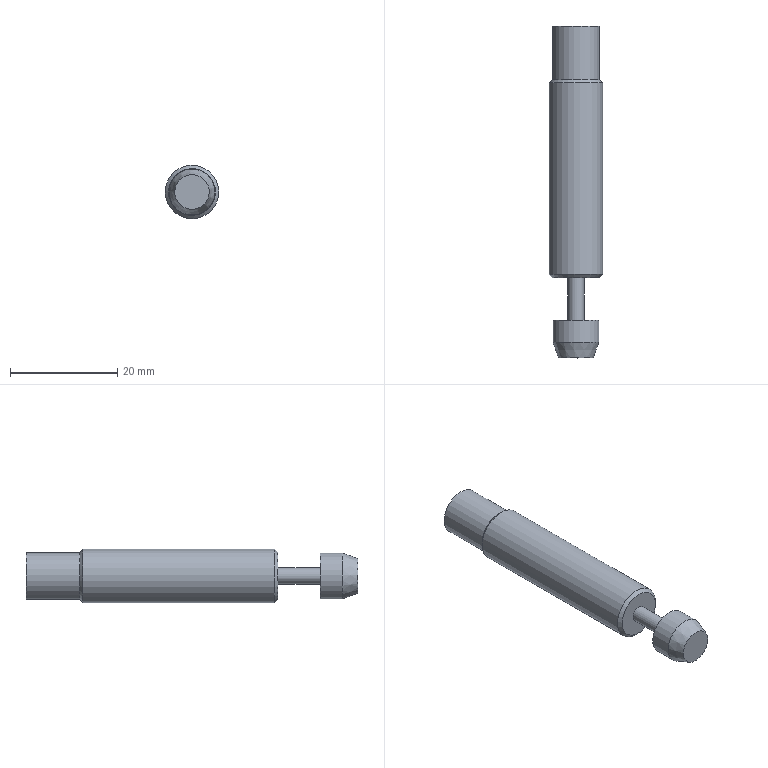Part | NX | features CYL_3 2 | 1 solid | 11 faces | box 10 x 62 x 10 mm | volume 3924 mm3 | cylinder 4 | plane 4 | cone 3 | commonest cylinder face diameters 3 x1 8.6 x1 8.773 x1 10 x1
STEP:
#1=CARTESIAN_POINT('',(-17.839,371.216,109.755));
#2=VERTEX_POINT('',#1);
#3=CARTESIAN_POINT('',(-17.5,371.216,105.381));
#4=DIRECTION('',(0.,-1.,0.));
#5=DIRECTION('',(-0.07719,0.,0.997));
#6=AXIS2_PLACEMENT_3D('',#3,#4,#5);
#7=CIRCLE('',#6,4.387);
#8=EDGE_CURVE('',#2,#2,#7,.T.);
#9=ORIENTED_EDGE('',*,*,#8,.T.);
#10=EDGE_LOOP('',(#9));
#11=FACE_BOUND('',#10,.T.);
#12=CARTESIAN_POINT('',(-17.839,361.216,109.755));
#13=VERTEX_POINT('',#12);
#14=CARTESIAN_POINT('',(-17.5,361.216,105.381));
#15=DIRECTION('',(0.,-1.,0.));
#16=DIRECTION('',(-0.07719,0.,0.997));
#17=AXIS2_PLACEMENT_3D('',#14,#15,#16);
#18=CIRCLE('',#17,4.386);
#19=EDGE_CURVE('',#13,#13,#18,.T.);
#20=ORIENTED_EDGE('',*,*,#19,.F.);
#21=EDGE_LOOP('',(#20));
#22=FACE_BOUND('',#21,.T.);
#23=CARTESIAN_POINT('',(-17.5,824.216,105.381));
#24=DIRECTION('',(0.,-1.,0.));
#25=DIRECTION('',(0.07719,0.,-0.997));
#26=AXIS2_PLACEMENT_3D('',#23,#24,#25);
#27=CYLINDRICAL_SURFACE('',#26,4.386);
#28=ADVANCED_FACE('',(#11,#22),#27,.T.);
#29=ORIENTED_EDGE('',*,*,#19,.T.);
#30=EDGE_LOOP('',(#29));
#31=FACE_BOUND('',#30,.T.);
#32=CARTESIAN_POINT('',(-17.886,360.602,110.366));
#33=VERTEX_POINT('',#32);
#34=CARTESIAN_POINT('',(-17.5,360.602,105.381));
#35=DIRECTION('',(0.,-1.,0.));
#36=DIRECTION('',(-0.07719,0.,0.997));
#37=AXIS2_PLACEMENT_3D('',#34,#35,#36);
#38=CIRCLE('',#37,5.);
#39=EDGE_CURVE('',#33,#33,#38,.T.);
#40=ORIENTED_EDGE('',*,*,#39,.F.);
#41=EDGE_LOOP('',(#40));
#42=FACE_BOUND('',#41,.T.);
#43=CARTESIAN_POINT('',(-17.5,361.216,105.381));
#44=DIRECTION('',(0.,-1.,0.));
#45=DIRECTION('',(0.07719,0.,-0.997));
#46=AXIS2_PLACEMENT_3D('',#43,#44,#45);
#47=CONICAL_SURFACE('',#46,4.386,0.7854);
#48=ADVANCED_FACE('',(#31,#42),#47,.T.);
#49=ORIENTED_EDGE('',*,*,#39,.T.);
#50=EDGE_LOOP('',(#49));
#51=FACE_BOUND('',#50,.T.);
#52=CARTESIAN_POINT('',(-17.886,324.829,110.366));
#53=VERTEX_POINT('',#52);
#54=CARTESIAN_POINT('',(-17.5,324.829,105.381));
#55=DIRECTION('',(0.,-1.,0.));
#56=DIRECTION('',(-0.07719,0.,0.997));
#57=AXIS2_PLACEMENT_3D('',#54,#55,#56);
#58=CIRCLE('',#57,5.);
#59=EDGE_CURVE('',#53,#53,#58,.T.);
#60=ORIENTED_EDGE('',*,*,#59,.F.);
#61=EDGE_LOOP('',(#60));
#62=FACE_BOUND('',#61,.T.);
#63=CARTESIAN_POINT('',(-17.5,824.216,105.381));
#64=DIRECTION('',(0.,-1.,0.));
#65=DIRECTION('',(0.07719,0.,-0.997));
#66=AXIS2_PLACEMENT_3D('',#63,#64,#65);
#67=CYLINDRICAL_SURFACE('',#66,5.);
#68=ADVANCED_FACE('',(#51,#62),#67,.T.);
#69=ORIENTED_EDGE('',*,*,#59,.T.);
#70=EDGE_LOOP('',(#69));
#71=FACE_BOUND('',#70,.T.);
#72=CARTESIAN_POINT('',(-17.839,324.216,109.755));
#73=VERTEX_POINT('',#72);
#74=CARTESIAN_POINT('',(-17.5,324.216,105.381));
#75=DIRECTION('',(0.,-1.,0.));
#76=DIRECTION('',(-0.07719,0.,0.997));
#77=AXIS2_PLACEMENT_3D('',#74,#75,#76);
#78=CIRCLE('',#77,4.386);
#79=EDGE_CURVE('',#73,#73,#78,.T.);
#80=ORIENTED_EDGE('',*,*,#79,.F.);
#81=EDGE_LOOP('',(#80));
#82=FACE_BOUND('',#81,.T.);
#83=CARTESIAN_POINT('',(-17.5,324.829,105.381));
#84=DIRECTION('',(0.,1.,0.));
#85=DIRECTION('',(-0.07719,0.,0.997));
#86=AXIS2_PLACEMENT_3D('',#83,#84,#85);
#87=CONICAL_SURFACE('',#86,5.,0.7854);
#88=ADVANCED_FACE('',(#71,#82),#87,.T.);
#89=CARTESIAN_POINT('',(-17.616,324.216,106.877));
#90=VERTEX_POINT('',#89);
#91=CARTESIAN_POINT('',(-17.5,324.216,105.381));
#92=DIRECTION('',(0.,-1.,0.));
#93=DIRECTION('',(-0.07719,0.,0.997));
#94=AXIS2_PLACEMENT_3D('',#91,#92,#93);
#95=CIRCLE('',#94,1.5);
#96=EDGE_CURVE('',#90,#90,#95,.T.);
#97=ORIENTED_EDGE('',*,*,#96,.T.);
#98=EDGE_LOOP('',(#97));
#99=FACE_BOUND('',#98,.T.);
#100=CARTESIAN_POINT('',(-17.616,316.216,106.877));
#101=VERTEX_POINT('',#100);
#102=CARTESIAN_POINT('',(-17.5,316.216,105.381));
#103=DIRECTION('',(0.,-1.,0.));
#104=DIRECTION('',(-0.07719,0.,0.997));
#105=AXIS2_PLACEMENT_3D('',#102,#103,#104);
#106=CIRCLE('',#105,1.5);
#107=EDGE_CURVE('',#101,#101,#106,.T.);
#108=ORIENTED_EDGE('',*,*,#107,.F.);
#109=EDGE_LOOP('',(#108));
#110=FACE_BOUND('',#109,.T.);
#111=CARTESIAN_POINT('',(-17.5,824.216,105.381));
#112=DIRECTION('',(0.,-1.,0.));
#113=DIRECTION('',(0.07719,0.,-0.997));
#114=AXIS2_PLACEMENT_3D('',#111,#112,#113);
#115=CYLINDRICAL_SURFACE('',#114,1.5);
#116=ADVANCED_FACE('',(#99,#110),#115,.T.);
#117=CARTESIAN_POINT('',(-17.832,316.216,109.668));
#118=VERTEX_POINT('',#117);
#119=CARTESIAN_POINT('',(-17.5,316.216,105.381));
#120=DIRECTION('',(0.,-1.,0.));
#121=DIRECTION('',(-0.07719,0.,0.997));
#122=AXIS2_PLACEMENT_3D('',#119,#120,#121);
#123=CIRCLE('',#122,4.3);
#124=EDGE_CURVE('',#118,#118,#123,.T.);
#125=ORIENTED_EDGE('',*,*,#124,.T.);
#126=EDGE_LOOP('',(#125));
#127=FACE_BOUND('',#126,.T.);
#128=CARTESIAN_POINT('',(-17.832,312.14,109.668));
#129=VERTEX_POINT('',#128);
#130=CARTESIAN_POINT('',(-17.5,312.14,105.381));
#131=DIRECTION('',(0.,-1.,0.));
#132=DIRECTION('',(-0.07719,0.,0.997));
#133=AXIS2_PLACEMENT_3D('',#130,#131,#132);
#134=CIRCLE('',#133,4.3);
#135=EDGE_CURVE('',#129,#129,#134,.T.);
#136=ORIENTED_EDGE('',*,*,#135,.F.);
#137=EDGE_LOOP('',(#136));
#138=FACE_BOUND('',#137,.T.);
#139=CARTESIAN_POINT('',(-17.5,824.216,105.381));
#140=DIRECTION('',(0.,-1.,0.));
#141=DIRECTION('',(0.07719,0.,-0.997));
#142=AXIS2_PLACEMENT_3D('',#139,#140,#141);
#143=CYLINDRICAL_SURFACE('',#142,4.3);
#144=ADVANCED_FACE('',(#127,#138),#143,.T.);
#145=ORIENTED_EDGE('',*,*,#135,.T.);
#146=EDGE_LOOP('',(#145));
#147=FACE_BOUND('',#146,.T.);
#148=CARTESIAN_POINT('',(-17.75,309.216,108.607));
#149=VERTEX_POINT('',#148);
#150=CARTESIAN_POINT('',(-17.5,309.216,105.381));
#151=DIRECTION('',(0.,-1.,0.));
#152=DIRECTION('',(-0.07719,0.,0.997));
#153=AXIS2_PLACEMENT_3D('',#150,#151,#152);
#154=CIRCLE('',#153,3.236);
#155=EDGE_CURVE('',#149,#149,#154,.T.);
#156=ORIENTED_EDGE('',*,*,#155,.F.);
#157=EDGE_LOOP('',(#156));
#158=FACE_BOUND('',#157,.T.);
#159=CARTESIAN_POINT('',(-17.5,312.14,105.381));
#160=DIRECTION('',(0.,1.,0.));
#161=DIRECTION('',(-0.07719,0.,0.997));
#162=AXIS2_PLACEMENT_3D('',#159,#160,#161);
#163=CONICAL_SURFACE('',#162,4.3,0.3491);
#164=ADVANCED_FACE('',(#147,#158),#163,.T.);
#165=ORIENTED_EDGE('',*,*,#155,.T.);
#166=EDGE_LOOP('',(#165));
#167=FACE_BOUND('',#166,.T.);
#168=CARTESIAN_POINT('',(-17.5,309.216,105.381));
#169=DIRECTION('',(0.,1.,0.));
#170=DIRECTION('',(-0.07719,0.,0.997));
#171=AXIS2_PLACEMENT_3D('',#168,#169,#170);
#172=PLANE('',#171);
#173=ADVANCED_FACE('',(#167),#172,.F.);
#174=ORIENTED_EDGE('',*,*,#124,.F.);
#175=EDGE_LOOP('',(#174));
#176=FACE_BOUND('',#175,.T.);
#177=ORIENTED_EDGE('',*,*,#107,.T.);
#178=EDGE_LOOP('',(#177));
#179=FACE_BOUND('',#178,.T.);
#180=CARTESIAN_POINT('',(-21.787,316.216,105.049));
#181=DIRECTION('',(0.,-1.,0.));
#182=DIRECTION('',(0.07719,0.,-0.997));
#183=AXIS2_PLACEMENT_3D('',#180,#181,#182);
#184=PLANE('',#183);
#185=ADVANCED_FACE('',(#176,#179),#184,.F.);
#186=ORIENTED_EDGE('',*,*,#96,.F.);
#187=EDGE_LOOP('',(#186));
#188=FACE_BOUND('',#187,.T.);
#189=ORIENTED_EDGE('',*,*,#79,.T.);
#190=EDGE_LOOP('',(#189));
#191=FACE_BOUND('',#190,.T.);
#192=CARTESIAN_POINT('',(-18.996,324.216,105.265));
#193=DIRECTION('',(0.,1.,0.));
#194=DIRECTION('',(-0.07719,0.,0.997));
#195=AXIS2_PLACEMENT_3D('',#192,#193,#194);
#196=PLANE('',#195);
#197=ADVANCED_FACE('',(#188,#191),#196,.F.);
#198=ORIENTED_EDGE('',*,*,#8,.F.);
#199=EDGE_LOOP('',(#198));
#200=FACE_BOUND('',#199,.T.);
#201=CARTESIAN_POINT('',(-21.873,371.216,105.043));
#202=DIRECTION('',(0.,-1.,0.));
#203=DIRECTION('',(0.07719,0.,-0.997));
#204=AXIS2_PLACEMENT_3D('',#201,#202,#203);
#205=PLANE('',#204);
#206=ADVANCED_FACE('',(#200),#205,.F.);
#207=CLOSED_SHELL('',(#28,#48,#68,#88,#116,#144,#164,#173,#185,#197,#206));
#208=MANIFOLD_SOLID_BREP('',#207);
#209=(LENGTH_UNIT()NAMED_UNIT(*)SI_UNIT(.MILLI.,.METRE.));
#210=UNCERTAINTY_MEASURE_WITH_UNIT(LENGTH_MEASURE(0.00001),#209,'','');
#211=(NAMED_UNIT(*)PLANE_ANGLE_UNIT()SI_UNIT($,.RADIAN.));
#212=(NAMED_UNIT(*)SI_UNIT($,.STERADIAN.)SOLID_ANGLE_UNIT());
#213=(GEOMETRIC_REPRESENTATION_CONTEXT(3)GLOBAL_UNCERTAINTY_ASSIGNED_CONTEXT((#210))GLOBAL_UNIT_ASSIGNED_CONTEXT((#209,#211,#212))REPRESENTATION_CONTEXT('',''));
#214=ADVANCED_BREP_SHAPE_REPRESENTATION('',(#208),#213);